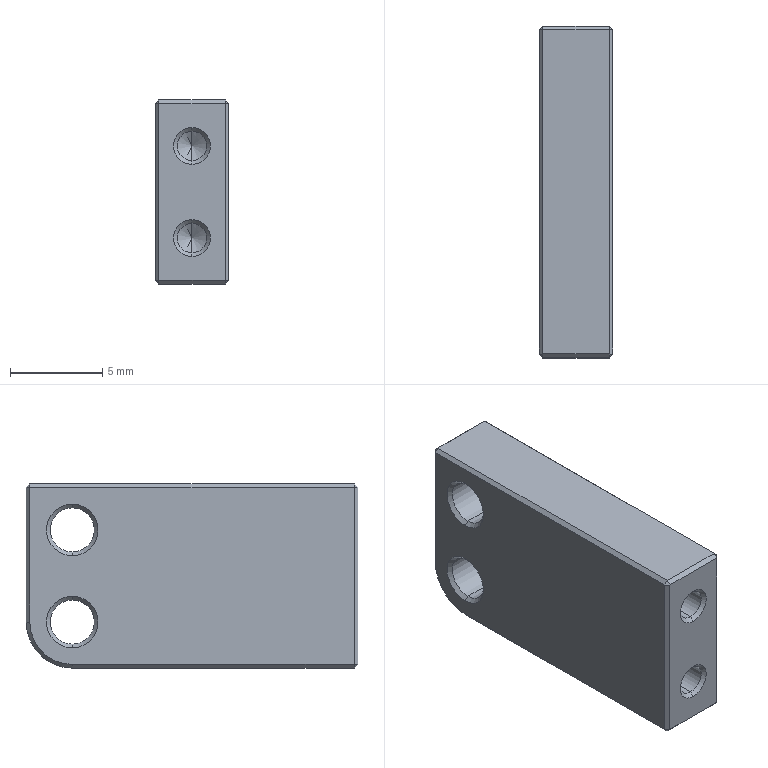Part | SolidWorks | features HoleWzd 2, Chamfer 1, Extrusion 1, Fillet 1 | 1 solid | 50 faces | box 4 x 18 x 10 mm | volume 638.389 mm3 | plane 23 | cone 18 | cylinder 9 | commonest cylinder face diameters 1.6 x4 2.4 x4 5 x1
STEP:
#1=CARTESIAN_POINT('',(0.2,15.5,-3.7));
#2=VERTEX_POINT('',#1);
#3=CARTESIAN_POINT('',(0.2,15.5,-1.3));
#4=VERTEX_POINT('',#3);
#5=CARTESIAN_POINT('',(0.2,15.5,-2.5));
#6=DIRECTION('',(-1.,0.,0.));
#7=DIRECTION('',(0.,0.,-1.));
#8=AXIS2_PLACEMENT_3D('',#5,#6,#7);
#9=CIRCLE('',#8,1.2);
#10=EDGE_CURVE('',#2,#4,#9,.T.);
#11=ORIENTED_EDGE('',*,*,#10,.F.);
#12=CARTESIAN_POINT('',(0.,15.5,-3.9));
#13=VERTEX_POINT('',#12);
#14=CARTESIAN_POINT('',(0.,15.5,-3.9));
#15=DIRECTION('',(-0.7071,0.,-0.7071));
#16=VECTOR('',#15,1000.);
#17=LINE('',#14,#16);
#18=EDGE_CURVE('',#2,#13,#17,.T.);
#19=ORIENTED_EDGE('',*,*,#18,.T.);
#20=CARTESIAN_POINT('',(0.,15.5,-1.1));
#21=VERTEX_POINT('',#20);
#22=CARTESIAN_POINT('',(0.,15.5,-2.5));
#23=DIRECTION('',(1.,0.,0.));
#24=DIRECTION('',(0.,0.,-1.));
#25=AXIS2_PLACEMENT_3D('',#22,#23,#24);
#26=CIRCLE('',#25,1.4);
#27=EDGE_CURVE('',#21,#13,#26,.T.);
#28=ORIENTED_EDGE('',*,*,#27,.F.);
#29=CARTESIAN_POINT('',(0.,15.5,-1.1));
#30=DIRECTION('',(-0.7071,0.,0.7071));
#31=VECTOR('',#30,1000.);
#32=LINE('',#29,#31);
#33=EDGE_CURVE('',#4,#21,#32,.T.);
#34=ORIENTED_EDGE('',*,*,#33,.F.);
#35=EDGE_LOOP('',(#11,#19,#28,#34));
#36=FACE_OUTER_BOUND('',#35,.T.);
#37=CARTESIAN_POINT('',(0.,15.5,-2.5));
#38=DIRECTION('',(-1.,0.,0.));
#39=DIRECTION('',(0.,0.,1.));
#40=AXIS2_PLACEMENT_3D('',#37,#38,#39);
#41=CONICAL_SURFACE('',#40,1.4,0.7854);
#42=ADVANCED_FACE('',(#36),#41,.F.);
#43=CARTESIAN_POINT('',(0.2,15.5,-8.7));
#44=VERTEX_POINT('',#43);
#45=CARTESIAN_POINT('',(0.2,15.5,-6.3));
#46=VERTEX_POINT('',#45);
#47=CARTESIAN_POINT('',(0.2,15.5,-7.5));
#48=DIRECTION('',(-1.,0.,0.));
#49=DIRECTION('',(0.,0.,-1.));
#50=AXIS2_PLACEMENT_3D('',#47,#48,#49);
#51=CIRCLE('',#50,1.2);
#52=EDGE_CURVE('',#44,#46,#51,.T.);
#53=ORIENTED_EDGE('',*,*,#52,.F.);
#54=CARTESIAN_POINT('',(0.,15.5,-8.9));
#55=VERTEX_POINT('',#54);
#56=CARTESIAN_POINT('',(0.,15.5,-8.9));
#57=DIRECTION('',(-0.7071,0.,-0.7071));
#58=VECTOR('',#57,1000.);
#59=LINE('',#56,#58);
#60=EDGE_CURVE('',#44,#55,#59,.T.);
#61=ORIENTED_EDGE('',*,*,#60,.T.);
#62=CARTESIAN_POINT('',(0.,15.5,-6.1));
#63=VERTEX_POINT('',#62);
#64=CARTESIAN_POINT('',(0.,15.5,-7.5));
#65=DIRECTION('',(1.,0.,0.));
#66=DIRECTION('',(0.,0.,-1.));
#67=AXIS2_PLACEMENT_3D('',#64,#65,#66);
#68=CIRCLE('',#67,1.4);
#69=EDGE_CURVE('',#63,#55,#68,.T.);
#70=ORIENTED_EDGE('',*,*,#69,.F.);
#71=CARTESIAN_POINT('',(0.,15.5,-6.1));
#72=DIRECTION('',(-0.7071,0.,0.7071));
#73=VECTOR('',#72,1000.);
#74=LINE('',#71,#73);
#75=EDGE_CURVE('',#46,#63,#74,.T.);
#76=ORIENTED_EDGE('',*,*,#75,.F.);
#77=EDGE_LOOP('',(#53,#61,#70,#76));
#78=FACE_OUTER_BOUND('',#77,.T.);
#79=CARTESIAN_POINT('',(0.,15.5,-7.5));
#80=DIRECTION('',(-1.,0.,0.));
#81=DIRECTION('',(0.,0.,1.));
#82=AXIS2_PLACEMENT_3D('',#79,#80,#81);
#83=CONICAL_SURFACE('',#82,1.4,0.7854);
#84=ADVANCED_FACE('',(#78),#83,.F.);
#85=CARTESIAN_POINT('',(2.,0.2,-1.7));
#86=VERTEX_POINT('',#85);
#87=CARTESIAN_POINT('',(2.,0.2,-3.3));
#88=VERTEX_POINT('',#87);
#89=CARTESIAN_POINT('',(2.,0.2,-2.5));
#90=DIRECTION('',(0.,-1.,0.));
#91=DIRECTION('',(0.,0.,-1.));
#92=AXIS2_PLACEMENT_3D('',#89,#90,#91);
#93=CIRCLE('',#92,0.8);
#94=EDGE_CURVE('',#86,#88,#93,.T.);
#95=ORIENTED_EDGE('',*,*,#94,.F.);
#96=CARTESIAN_POINT('',(2.,0.,-1.5));
#97=VERTEX_POINT('',#96);
#98=CARTESIAN_POINT('',(2.,0.2,-1.7));
#99=DIRECTION('',(0.,-0.7071,0.7071));
#100=VECTOR('',#99,1000.);
#101=LINE('',#98,#100);
#102=EDGE_CURVE('',#86,#97,#101,.T.);
#103=ORIENTED_EDGE('',*,*,#102,.T.);
#104=CARTESIAN_POINT('',(2.,0.,-3.5));
#105=VERTEX_POINT('',#104);
#106=CARTESIAN_POINT('',(2.,0.,-2.5));
#107=DIRECTION('',(0.,1.,0.));
#108=DIRECTION('',(0.,0.,-1.));
#109=AXIS2_PLACEMENT_3D('',#106,#107,#108);
#110=CIRCLE('',#109,1.);
#111=EDGE_CURVE('',#105,#97,#110,.T.);
#112=ORIENTED_EDGE('',*,*,#111,.F.);
#113=CARTESIAN_POINT('',(2.,0.2,-3.3));
#114=DIRECTION('',(0.,-0.7071,-0.7071));
#115=VECTOR('',#114,1000.);
#116=LINE('',#113,#115);
#117=EDGE_CURVE('',#88,#105,#116,.T.);
#118=ORIENTED_EDGE('',*,*,#117,.F.);
#119=EDGE_LOOP('',(#95,#103,#112,#118));
#120=FACE_OUTER_BOUND('',#119,.T.);
#121=CARTESIAN_POINT('',(2.,0.2,-2.5));
#122=DIRECTION('',(0.,-1.,0.));
#123=DIRECTION('',(0.,0.,-1.));
#124=AXIS2_PLACEMENT_3D('',#121,#122,#123);
#125=CONICAL_SURFACE('',#124,0.8,0.7854);
#126=ADVANCED_FACE('',(#120),#125,.F.);
#127=CARTESIAN_POINT('',(2.,0.2,-6.7));
#128=VERTEX_POINT('',#127);
#129=CARTESIAN_POINT('',(2.,0.2,-8.3));
#130=VERTEX_POINT('',#129);
#131=CARTESIAN_POINT('',(2.,0.2,-7.5));
#132=DIRECTION('',(0.,-1.,0.));
#133=DIRECTION('',(0.,0.,-1.));
#134=AXIS2_PLACEMENT_3D('',#131,#132,#133);
#135=CIRCLE('',#134,0.8);
#136=EDGE_CURVE('',#128,#130,#135,.T.);
#137=ORIENTED_EDGE('',*,*,#136,.F.);
#138=CARTESIAN_POINT('',(2.,0.,-6.5));
#139=VERTEX_POINT('',#138);
#140=CARTESIAN_POINT('',(2.,0.2,-6.7));
#141=DIRECTION('',(0.,-0.7071,0.7071));
#142=VECTOR('',#141,1000.);
#143=LINE('',#140,#142);
#144=EDGE_CURVE('',#128,#139,#143,.T.);
#145=ORIENTED_EDGE('',*,*,#144,.T.);
#146=CARTESIAN_POINT('',(2.,0.,-8.5));
#147=VERTEX_POINT('',#146);
#148=CARTESIAN_POINT('',(2.,0.,-7.5));
#149=DIRECTION('',(0.,1.,0.));
#150=DIRECTION('',(0.,0.,-1.));
#151=AXIS2_PLACEMENT_3D('',#148,#149,#150);
#152=CIRCLE('',#151,1.);
#153=EDGE_CURVE('',#147,#139,#152,.T.);
#154=ORIENTED_EDGE('',*,*,#153,.F.);
#155=CARTESIAN_POINT('',(2.,0.2,-8.3));
#156=DIRECTION('',(0.,-0.7071,-0.7071));
#157=VECTOR('',#156,1000.);
#158=LINE('',#155,#157);
#159=EDGE_CURVE('',#130,#147,#158,.T.);
#160=ORIENTED_EDGE('',*,*,#159,.F.);
#161=EDGE_LOOP('',(#137,#145,#154,#160));
#162=FACE_OUTER_BOUND('',#161,.T.);
#163=CARTESIAN_POINT('',(2.,0.2,-7.5));
#164=DIRECTION('',(0.,-1.,0.));
#165=DIRECTION('',(0.,0.,-1.));
#166=AXIS2_PLACEMENT_3D('',#163,#164,#165);
#167=CONICAL_SURFACE('',#166,0.8,0.7854);
#168=ADVANCED_FACE('',(#162),#167,.F.);
#169=CARTESIAN_POINT('',(2.,6.4,-1.7));
#170=VERTEX_POINT('',#169);
#171=CARTESIAN_POINT('',(2.,6.4,-3.3));
#172=VERTEX_POINT('',#171);
#173=CARTESIAN_POINT('',(2.,6.4,-2.5));
#174=DIRECTION('',(0.,-1.,0.));
#175=DIRECTION('',(0.,0.,-1.));
#176=AXIS2_PLACEMENT_3D('',#173,#174,#175);
#177=CIRCLE('',#176,0.8);
#178=EDGE_CURVE('',#170,#172,#177,.T.);
#179=ORIENTED_EDGE('',*,*,#178,.F.);
#180=CARTESIAN_POINT('',(2.,0.,-1.7));
#181=DIRECTION('',(0.,-1.,0.));
#182=VECTOR('',#181,1000.);
#183=LINE('',#180,#182);
#184=EDGE_CURVE('',#170,#86,#183,.T.);
#185=ORIENTED_EDGE('',*,*,#184,.T.);
#186=ORIENTED_EDGE('',*,*,#94,.T.);
#187=CARTESIAN_POINT('',(2.,0.,-3.3));
#188=DIRECTION('',(0.,-1.,0.));
#189=VECTOR('',#188,1000.);
#190=LINE('',#187,#189);
#191=EDGE_CURVE('',#172,#88,#190,.T.);
#192=ORIENTED_EDGE('',*,*,#191,.F.);
#193=EDGE_LOOP('',(#179,#185,#186,#192));
#194=FACE_OUTER_BOUND('',#193,.T.);
#195=CARTESIAN_POINT('',(2.,0.,-2.5));
#196=DIRECTION('',(0.,-1.,0.));
#197=DIRECTION('',(0.,0.,-1.));
#198=AXIS2_PLACEMENT_3D('',#195,#196,#197);
#199=CYLINDRICAL_SURFACE('',#198,0.8);
#200=ADVANCED_FACE('',(#194),#199,.F.);
#201=CARTESIAN_POINT('',(2.,6.881,-2.5));
#202=VERTEX_POINT('',#201);
#203=CARTESIAN_POINT('',(2.,6.4,-3.3));
#204=DIRECTION('',(0.,-0.515,-0.8572));
#205=VECTOR('',#204,1000.);
#206=LINE('',#203,#205);
#207=EDGE_CURVE('',#202,#172,#206,.T.);
#208=ORIENTED_EDGE('',*,*,#207,.F.);
#209=CARTESIAN_POINT('',(2.,6.4,-1.7));
#210=DIRECTION('',(0.,-0.515,0.8572));
#211=VECTOR('',#210,1000.);
#212=LINE('',#209,#211);
#213=EDGE_CURVE('',#202,#170,#212,.T.);
#214=ORIENTED_EDGE('',*,*,#213,.T.);
#215=ORIENTED_EDGE('',*,*,#178,.T.);
#216=EDGE_LOOP('',(#208,#214,#215));
#217=FACE_OUTER_BOUND('',#216,.T.);
#218=CARTESIAN_POINT('',(2.,6.4,-2.5));
#219=DIRECTION('',(0.,-1.,0.));
#220=DIRECTION('',(0.,0.,-1.));
#221=AXIS2_PLACEMENT_3D('',#218,#219,#220);
#222=CONICAL_SURFACE('',#221,0.8,1.03);
#223=ADVANCED_FACE('',(#217),#222,.F.);
#224=CARTESIAN_POINT('',(2.,6.4,-6.7));
#225=VERTEX_POINT('',#224);
#226=CARTESIAN_POINT('',(2.,6.4,-8.3));
#227=VERTEX_POINT('',#226);
#228=CARTESIAN_POINT('',(2.,6.4,-7.5));
#229=DIRECTION('',(0.,-1.,0.));
#230=DIRECTION('',(0.,0.,-1.));
#231=AXIS2_PLACEMENT_3D('',#228,#229,#230);
#232=CIRCLE('',#231,0.8);
#233=EDGE_CURVE('',#225,#227,#232,.T.);
#234=ORIENTED_EDGE('',*,*,#233,.F.);
#235=CARTESIAN_POINT('',(2.,0.,-6.7));
#236=DIRECTION('',(0.,-1.,0.));
#237=VECTOR('',#236,1000.);
#238=LINE('',#235,#237);
#239=EDGE_CURVE('',#225,#128,#238,.T.);
#240=ORIENTED_EDGE('',*,*,#239,.T.);
#241=ORIENTED_EDGE('',*,*,#136,.T.);
#242=CARTESIAN_POINT('',(2.,0.,-8.3));
#243=DIRECTION('',(0.,-1.,0.));
#244=VECTOR('',#243,1000.);
#245=LINE('',#242,#244);
#246=EDGE_CURVE('',#227,#130,#245,.T.);
#247=ORIENTED_EDGE('',*,*,#246,.F.);
#248=EDGE_LOOP('',(#234,#240,#241,#247));
#249=FACE_OUTER_BOUND('',#248,.T.);
#250=CARTESIAN_POINT('',(2.,0.,-7.5));
#251=DIRECTION('',(0.,-1.,0.));
#252=DIRECTION('',(0.,0.,-1.));
#253=AXIS2_PLACEMENT_3D('',#250,#251,#252);
#254=CYLINDRICAL_SURFACE('',#253,0.8);
#255=ADVANCED_FACE('',(#249),#254,.F.);
#256=CARTESIAN_POINT('',(2.,6.881,-7.5));
#257=VERTEX_POINT('',#256);
#258=CARTESIAN_POINT('',(2.,6.4,-8.3));
#259=DIRECTION('',(0.,-0.515,-0.8572));
#260=VECTOR('',#259,1000.);
#261=LINE('',#258,#260);
#262=EDGE_CURVE('',#257,#227,#261,.T.);
#263=ORIENTED_EDGE('',*,*,#262,.F.);
#264=CARTESIAN_POINT('',(2.,6.4,-6.7));
#265=DIRECTION('',(0.,-0.515,0.8572));
#266=VECTOR('',#265,1000.);
#267=LINE('',#264,#266);
#268=EDGE_CURVE('',#257,#225,#267,.T.);
#269=ORIENTED_EDGE('',*,*,#268,.T.);
#270=ORIENTED_EDGE('',*,*,#233,.T.);
#271=EDGE_LOOP('',(#263,#269,#270));
#272=FACE_OUTER_BOUND('',#271,.T.);
#273=CARTESIAN_POINT('',(2.,6.4,-7.5));
#274=DIRECTION('',(0.,-1.,0.));
#275=DIRECTION('',(0.,0.,-1.));
#276=AXIS2_PLACEMENT_3D('',#273,#274,#275);
#277=CONICAL_SURFACE('',#276,0.8,1.03);
#278=ADVANCED_FACE('',(#272),#277,.F.);
#279=CARTESIAN_POINT('',(2.95,15.5,-1.3));
#280=VERTEX_POINT('',#279);
#281=CARTESIAN_POINT('',(2.95,15.5,-3.7));
#282=VERTEX_POINT('',#281);
#283=CARTESIAN_POINT('',(2.95,15.5,-2.5));
#284=DIRECTION('',(1.,0.,0.));
#285=DIRECTION('',(0.,0.,-1.));
#286=AXIS2_PLACEMENT_3D('',#283,#284,#285);
#287=CIRCLE('',#286,1.2);
#288=EDGE_CURVE('',#280,#282,#287,.T.);
#289=ORIENTED_EDGE('',*,*,#288,.F.);
#290=CARTESIAN_POINT('',(4.,15.5,-0.25));
#291=VERTEX_POINT('',#290);
#292=CARTESIAN_POINT('',(4.,15.5,-0.25));
#293=DIRECTION('',(0.7071,0.,0.7071));
#294=VECTOR('',#293,1000.);
#295=LINE('',#292,#294);
#296=EDGE_CURVE('',#280,#291,#295,.T.);
#297=ORIENTED_EDGE('',*,*,#296,.T.);
#298=CARTESIAN_POINT('',(4.,15.5,-4.75));
#299=VERTEX_POINT('',#298);
#300=CARTESIAN_POINT('',(4.,15.5,-2.5));
#301=DIRECTION('',(1.,0.,0.));
#302=DIRECTION('',(0.,0.,-1.));
#303=AXIS2_PLACEMENT_3D('',#300,#301,#302);
#304=CIRCLE('',#303,2.25);
#305=EDGE_CURVE('',#291,#299,#304,.T.);
#306=ORIENTED_EDGE('',*,*,#305,.T.);
#307=CARTESIAN_POINT('',(4.,15.5,-4.75));
#308=DIRECTION('',(0.7071,0.,-0.7071));
#309=VECTOR('',#308,1000.);
#310=LINE('',#307,#309);
#311=EDGE_CURVE('',#282,#299,#310,.T.);
#312=ORIENTED_EDGE('',*,*,#311,.F.);
#313=EDGE_LOOP('',(#289,#297,#306,#312));
#314=FACE_OUTER_BOUND('',#313,.T.);
#315=CARTESIAN_POINT('',(4.,15.5,-2.5));
#316=DIRECTION('',(1.,0.,0.));
#317=DIRECTION('',(0.,0.,-1.));
#318=AXIS2_PLACEMENT_3D('',#315,#316,#317);
#319=CONICAL_SURFACE('',#318,2.25,0.7854);
#320=ADVANCED_FACE('',(#314),#319,.F.);
#321=ORIENTED_EDGE('',*,*,#10,.T.);
#322=CARTESIAN_POINT('',(4.,15.5,-1.3));
#323=DIRECTION('',(1.,0.,0.));
#324=VECTOR('',#323,1000.);
#325=LINE('',#322,#324);
#326=EDGE_CURVE('',#4,#280,#325,.T.);
#327=ORIENTED_EDGE('',*,*,#326,.T.);
#328=ORIENTED_EDGE('',*,*,#288,.T.);
#329=CARTESIAN_POINT('',(4.,15.5,-3.7));
#330=DIRECTION('',(1.,0.,0.));
#331=VECTOR('',#330,1000.);
#332=LINE('',#329,#331);
#333=EDGE_CURVE('',#2,#282,#332,.T.);
#334=ORIENTED_EDGE('',*,*,#333,.F.);
#335=EDGE_LOOP('',(#321,#327,#328,#334));
#336=FACE_OUTER_BOUND('',#335,.T.);
#337=CARTESIAN_POINT('',(4.,15.5,-2.5));
#338=DIRECTION('',(1.,0.,0.));
#339=DIRECTION('',(0.,0.,-1.));
#340=AXIS2_PLACEMENT_3D('',#337,#338,#339);
#341=CYLINDRICAL_SURFACE('',#340,1.2);
#342=ADVANCED_FACE('',(#336),#341,.F.);
#343=CARTESIAN_POINT('',(2.95,15.5,-6.3));
#344=VERTEX_POINT('',#343);
#345=CARTESIAN_POINT('',(2.95,15.5,-8.7));
#346=VERTEX_POINT('',#345);
#347=CARTESIAN_POINT('',(2.95,15.5,-7.5));
#348=DIRECTION('',(1.,0.,0.));
#349=DIRECTION('',(0.,0.,-1.));
#350=AXIS2_PLACEMENT_3D('',#347,#348,#349);
#351=CIRCLE('',#350,1.2);
#352=EDGE_CURVE('',#344,#346,#351,.T.);
#353=ORIENTED_EDGE('',*,*,#352,.F.);
#354=CARTESIAN_POINT('',(4.,15.5,-5.25));
#355=VERTEX_POINT('',#354);
#356=CARTESIAN_POINT('',(4.,15.5,-5.25));
#357=DIRECTION('',(0.7071,0.,0.7071));
#358=VECTOR('',#357,1000.);
#359=LINE('',#356,#358);
#360=EDGE_CURVE('',#344,#355,#359,.T.);
#361=ORIENTED_EDGE('',*,*,#360,.T.);
#362=CARTESIAN_POINT('',(4.,15.5,-9.75));
#363=VERTEX_POINT('',#362);
#364=CARTESIAN_POINT('',(4.,15.5,-7.5));
#365=DIRECTION('',(1.,0.,0.));
#366=DIRECTION('',(0.,0.,-1.));
#367=AXIS2_PLACEMENT_3D('',#364,#365,#366);
#368=CIRCLE('',#367,2.25);
#369=EDGE_CURVE('',#355,#363,#368,.T.);
#370=ORIENTED_EDGE('',*,*,#369,.T.);
#371=CARTESIAN_POINT('',(4.,15.5,-9.75));
#372=DIRECTION('',(0.7071,0.,-0.7071));
#373=VECTOR('',#372,1000.);
#374=LINE('',#371,#373);
#375=EDGE_CURVE('',#346,#363,#374,.T.);
#376=ORIENTED_EDGE('',*,*,#375,.F.);
#377=EDGE_LOOP('',(#353,#361,#370,#376));
#378=FACE_OUTER_BOUND('',#377,.T.);
#379=CARTESIAN_POINT('',(4.,15.5,-7.5));
#380=DIRECTION('',(1.,0.,0.));
#381=DIRECTION('',(0.,0.,-1.));
#382=AXIS2_PLACEMENT_3D('',#379,#380,#381);
#383=CONICAL_SURFACE('',#382,2.25,0.7854);
#384=ADVANCED_FACE('',(#378),#383,.F.);
#385=ORIENTED_EDGE('',*,*,#52,.T.);
#386=CARTESIAN_POINT('',(4.,15.5,-6.3));
#387=DIRECTION('',(1.,0.,0.));
#388=VECTOR('',#387,1000.);
#389=LINE('',#386,#388);
#390=EDGE_CURVE('',#46,#344,#389,.T.);
#391=ORIENTED_EDGE('',*,*,#390,.T.);
#392=ORIENTED_EDGE('',*,*,#352,.T.);
#393=CARTESIAN_POINT('',(4.,15.5,-8.7));
#394=DIRECTION('',(1.,0.,0.));
#395=VECTOR('',#394,1000.);
#396=LINE('',#393,#395);
#397=EDGE_CURVE('',#44,#346,#396,.T.);
#398=ORIENTED_EDGE('',*,*,#397,.F.);
#399=EDGE_LOOP('',(#385,#391,#392,#398));
#400=FACE_OUTER_BOUND('',#399,.T.);
#401=CARTESIAN_POINT('',(4.,15.5,-7.5));
#402=DIRECTION('',(1.,0.,0.));
#403=DIRECTION('',(0.,0.,-1.));
#404=AXIS2_PLACEMENT_3D('',#401,#402,#403);
#405=CYLINDRICAL_SURFACE('',#404,1.2);
#406=ADVANCED_FACE('',(#400),#405,.F.);
#407=CARTESIAN_POINT('',(4.,0.2,-0.2));
#408=VERTEX_POINT('',#407);
#409=CARTESIAN_POINT('',(4.,0.2,-9.8));
#410=VERTEX_POINT('',#409);
#411=CARTESIAN_POINT('',(4.,0.2,-10.));
#412=DIRECTION('',(0.,0.,-1.));
#413=VECTOR('',#412,1000.);
#414=LINE('',#411,#413);
#415=EDGE_CURVE('',#408,#410,#414,.T.);
#416=ORIENTED_EDGE('',*,*,#415,.T.);
#417=CARTESIAN_POINT('',(4.,15.5,-9.8));
#418=VERTEX_POINT('',#417);
#419=CARTESIAN_POINT('',(4.,18.,-9.8));
#420=DIRECTION('',(0.,1.,0.));
#421=VECTOR('',#420,1000.);
#422=LINE('',#419,#421);
#423=EDGE_CURVE('',#410,#418,#422,.T.);
#424=ORIENTED_EDGE('',*,*,#423,.T.);
#425=CARTESIAN_POINT('',(4.,17.8,-7.5));
#426=VERTEX_POINT('',#425);
#427=CARTESIAN_POINT('',(4.,15.5,-7.5));
#428=DIRECTION('',(1.,0.,0.));
#429=DIRECTION('',(0.,0.,1.));
#430=AXIS2_PLACEMENT_3D('',#427,#428,#429);
#431=CIRCLE('',#430,2.3);
#432=EDGE_CURVE('',#418,#426,#431,.T.);
#433=ORIENTED_EDGE('',*,*,#432,.T.);
#434=CARTESIAN_POINT('',(4.,17.8,-0.2));
#435=VERTEX_POINT('',#434);
#436=CARTESIAN_POINT('',(4.,17.8,0.));
#437=DIRECTION('',(0.,0.,1.));
#438=VECTOR('',#437,1000.);
#439=LINE('',#436,#438);
#440=EDGE_CURVE('',#426,#435,#439,.T.);
#441=ORIENTED_EDGE('',*,*,#440,.T.);
#442=CARTESIAN_POINT('',(4.,18.,-0.2));
#443=DIRECTION('',(0.,-1.,0.));
#444=VECTOR('',#443,1000.);
#445=LINE('',#442,#444);
#446=EDGE_CURVE('',#435,#408,#445,.T.);
#447=ORIENTED_EDGE('',*,*,#446,.T.);
#448=EDGE_LOOP('',(#416,#424,#433,#441,#447));
#449=FACE_OUTER_BOUND('',#448,.T.);
#450=CARTESIAN_POINT('',(4.,15.5,-2.5));
#451=DIRECTION('',(1.,0.,0.));
#452=DIRECTION('',(0.,0.,-1.));
#453=AXIS2_PLACEMENT_3D('',#450,#451,#452);
#454=CIRCLE('',#453,2.25);
#455=EDGE_CURVE('',#299,#291,#454,.T.);
#456=ORIENTED_EDGE('',*,*,#455,.F.);
#457=ORIENTED_EDGE('',*,*,#305,.F.);
#458=EDGE_LOOP('',(#456,#457));
#459=FACE_BOUND('',#458,.T.);
#460=CARTESIAN_POINT('',(4.,15.5,-7.5));
#461=DIRECTION('',(1.,0.,0.));
#462=DIRECTION('',(0.,0.,-1.));
#463=AXIS2_PLACEMENT_3D('',#460,#461,#462);
#464=CIRCLE('',#463,2.25);
#465=EDGE_CURVE('',#363,#355,#464,.T.);
#466=ORIENTED_EDGE('',*,*,#465,.F.);
#467=ORIENTED_EDGE('',*,*,#369,.F.);
#468=EDGE_LOOP('',(#466,#467));
#469=FACE_BOUND('',#468,.T.);
#470=CARTESIAN_POINT('',(4.,18.,0.));
#471=DIRECTION('',(-1.,0.,0.));
#472=DIRECTION('',(0.,0.,1.));
#473=AXIS2_PLACEMENT_3D('',#470,#471,#472);
#474=PLANE('',#473);
#475=ADVANCED_FACE('',(#449,#459,#469),#474,.F.);
#476=CARTESIAN_POINT('',(0.,0.2,-9.8));
#477=VERTEX_POINT('',#476);
#478=CARTESIAN_POINT('',(0.,0.2,-0.2));
#479=VERTEX_POINT('',#478);
#480=CARTESIAN_POINT('',(0.,0.2,0.));
#481=DIRECTION('',(0.,0.,1.));
#482=VECTOR('',#481,1000.);
#483=LINE('',#480,#482);
#484=EDGE_CURVE('',#477,#479,#483,.T.);
#485=ORIENTED_EDGE('',*,*,#484,.T.);
#486=CARTESIAN_POINT('',(0.,17.8,-0.2));
#487=VERTEX_POINT('',#486);
#488=CARTESIAN_POINT('',(0.,18.,-0.2));
#489=DIRECTION('',(0.,1.,0.));
#490=VECTOR('',#489,1000.);
#491=LINE('',#488,#490);
#492=EDGE_CURVE('',#479,#487,#491,.T.);
#493=ORIENTED_EDGE('',*,*,#492,.T.);
#494=CARTESIAN_POINT('',(0.,17.8,-7.5));
#495=VERTEX_POINT('',#494);
#496=CARTESIAN_POINT('',(0.,17.8,0.));
#497=DIRECTION('',(0.,0.,-1.));
#498=VECTOR('',#497,1000.);
#499=LINE('',#496,#498);
#500=EDGE_CURVE('',#487,#495,#499,.T.);
#501=ORIENTED_EDGE('',*,*,#500,.T.);
#502=CARTESIAN_POINT('',(0.,15.5,-9.8));
#503=VERTEX_POINT('',#502);
#504=CARTESIAN_POINT('',(0.,15.5,-7.5));
#505=DIRECTION('',(-1.,0.,0.));
#506=DIRECTION('',(0.,0.,-1.));
#507=AXIS2_PLACEMENT_3D('',#504,#505,#506);
#508=CIRCLE('',#507,2.3);
#509=EDGE_CURVE('',#495,#503,#508,.T.);
#510=ORIENTED_EDGE('',*,*,#509,.T.);
#511=CARTESIAN_POINT('',(0.,18.,-9.8));
#512=DIRECTION('',(0.,-1.,0.));
#513=VECTOR('',#512,1000.);
#514=LINE('',#511,#513);
#515=EDGE_CURVE('',#503,#477,#514,.T.);
#516=ORIENTED_EDGE('',*,*,#515,.T.);
#517=EDGE_LOOP('',(#485,#493,#501,#510,#516));
#518=FACE_OUTER_BOUND('',#517,.T.);
#519=ORIENTED_EDGE('',*,*,#69,.T.);
#520=CARTESIAN_POINT('',(0.,15.5,-7.5));
#521=DIRECTION('',(1.,0.,0.));
#522=DIRECTION('',(0.,0.,-1.));
#523=AXIS2_PLACEMENT_3D('',#520,#521,#522);
#524=CIRCLE('',#523,1.4);
#525=EDGE_CURVE('',#55,#63,#524,.T.);
#526=ORIENTED_EDGE('',*,*,#525,.T.);
#527=EDGE_LOOP('',(#519,#526));
#528=FACE_BOUND('',#527,.T.);
#529=ORIENTED_EDGE('',*,*,#27,.T.);
#530=CARTESIAN_POINT('',(0.,15.5,-2.5));
#531=DIRECTION('',(1.,0.,0.));
#532=DIRECTION('',(0.,0.,-1.));
#533=AXIS2_PLACEMENT_3D('',#530,#531,#532);
#534=CIRCLE('',#533,1.4);
#535=EDGE_CURVE('',#13,#21,#534,.T.);
#536=ORIENTED_EDGE('',*,*,#535,.T.);
#537=EDGE_LOOP('',(#529,#536));
#538=FACE_BOUND('',#537,.T.);
#539=CARTESIAN_POINT('',(0.,18.,0.));
#540=DIRECTION('',(1.,0.,0.));
#541=DIRECTION('',(0.,0.,-1.));
#542=AXIS2_PLACEMENT_3D('',#539,#540,#541);
#543=PLANE('',#542);
#544=ADVANCED_FACE('',(#518,#528,#538),#543,.F.);
#545=CARTESIAN_POINT('',(3.8,0.2,0.));
#546=VERTEX_POINT('',#545);
#547=CARTESIAN_POINT('',(3.8,17.8,0.));
#548=VERTEX_POINT('',#547);
#549=CARTESIAN_POINT('',(3.8,18.,0.));
#550=DIRECTION('',(0.,1.,0.));
#551=VECTOR('',#550,1000.);
#552=LINE('',#549,#551);
#553=EDGE_CURVE('',#546,#548,#552,.T.);
#554=ORIENTED_EDGE('',*,*,#553,.T.);
#555=CARTESIAN_POINT('',(0.2,17.8,0.));
#556=VERTEX_POINT('',#555);
#557=CARTESIAN_POINT('',(0.,17.8,0.));
#558=DIRECTION('',(-1.,0.,0.));
#559=VECTOR('',#558,1000.);
#560=LINE('',#557,#559);
#561=EDGE_CURVE('',#548,#556,#560,.T.);
#562=ORIENTED_EDGE('',*,*,#561,.T.);
#563=CARTESIAN_POINT('',(0.2,0.2,0.));
#564=VERTEX_POINT('',#563);
#565=CARTESIAN_POINT('',(0.2,18.,0.));
#566=DIRECTION('',(0.,-1.,0.));
#567=VECTOR('',#566,1000.);
#568=LINE('',#565,#567);
#569=EDGE_CURVE('',#556,#564,#568,.T.);
#570=ORIENTED_EDGE('',*,*,#569,.T.);
#571=CARTESIAN_POINT('',(4.,0.2,0.));
#572=DIRECTION('',(1.,0.,0.));
#573=VECTOR('',#572,1000.);
#574=LINE('',#571,#573);
#575=EDGE_CURVE('',#564,#546,#574,.T.);
#576=ORIENTED_EDGE('',*,*,#575,.T.);
#577=EDGE_LOOP('',(#554,#562,#570,#576));
#578=FACE_OUTER_BOUND('',#577,.T.);
#579=CARTESIAN_POINT('',(0.,18.,0.));
#580=DIRECTION('',(0.,0.,-1.));
#581=DIRECTION('',(-1.,0.,0.));
#582=AXIS2_PLACEMENT_3D('',#579,#580,#581);
#583=PLANE('',#582);
#584=ADVANCED_FACE('',(#578),#583,.F.);
#585=CARTESIAN_POINT('',(0.2,15.5,-10.));
#586=VERTEX_POINT('',#585);
#587=CARTESIAN_POINT('',(3.8,15.5,-10.));
#588=VERTEX_POINT('',#587);
#589=CARTESIAN_POINT('',(0.,15.5,-10.));
#590=DIRECTION('',(1.,0.,0.));
#591=VECTOR('',#590,1000.);
#592=LINE('',#589,#591);
#593=EDGE_CURVE('',#586,#588,#592,.T.);
#594=ORIENTED_EDGE('',*,*,#593,.T.);
#595=CARTESIAN_POINT('',(3.8,0.2,-10.));
#596=VERTEX_POINT('',#595);
#597=CARTESIAN_POINT('',(3.8,18.,-10.));
#598=DIRECTION('',(0.,-1.,0.));
#599=VECTOR('',#598,1000.);
#600=LINE('',#597,#599);
#601=EDGE_CURVE('',#588,#596,#600,.T.);
#602=ORIENTED_EDGE('',*,*,#601,.T.);
#603=CARTESIAN_POINT('',(0.2,0.2,-10.));
#604=VERTEX_POINT('',#603);
#605=CARTESIAN_POINT('',(0.,0.2,-10.));
#606=DIRECTION('',(-1.,0.,0.));
#607=VECTOR('',#606,1000.);
#608=LINE('',#605,#607);
#609=EDGE_CURVE('',#596,#604,#608,.T.);
#610=ORIENTED_EDGE('',*,*,#609,.T.);
#611=CARTESIAN_POINT('',(0.2,18.,-10.));
#612=DIRECTION('',(0.,1.,0.));
#613=VECTOR('',#612,1000.);
#614=LINE('',#611,#613);
#615=EDGE_CURVE('',#604,#586,#614,.T.);
#616=ORIENTED_EDGE('',*,*,#615,.T.);
#617=EDGE_LOOP('',(#594,#602,#610,#616));
#618=FACE_OUTER_BOUND('',#617,.T.);
#619=CARTESIAN_POINT('',(0.,18.,-10.));
#620=DIRECTION('',(0.,0.,1.));
#621=DIRECTION('',(1.,0.,0.));
#622=AXIS2_PLACEMENT_3D('',#619,#620,#621);
#623=PLANE('',#622);
#624=ADVANCED_FACE('',(#618),#623,.F.);
#625=CARTESIAN_POINT('',(0.2,18.,-0.2));
#626=VERTEX_POINT('',#625);
#627=CARTESIAN_POINT('',(3.8,18.,-0.2));
#628=VERTEX_POINT('',#627);
#629=CARTESIAN_POINT('',(0.,18.,-0.2));
#630=DIRECTION('',(1.,0.,0.));
#631=VECTOR('',#630,1000.);
#632=LINE('',#629,#631);
#633=EDGE_CURVE('',#626,#628,#632,.T.);
#634=ORIENTED_EDGE('',*,*,#633,.T.);
#635=CARTESIAN_POINT('',(3.8,18.,-7.5));
#636=VERTEX_POINT('',#635);
#637=CARTESIAN_POINT('',(3.8,18.,0.));
#638=DIRECTION('',(0.,0.,-1.));
#639=VECTOR('',#638,1000.);
#640=LINE('',#637,#639);
#641=EDGE_CURVE('',#628,#636,#640,.T.);
#642=ORIENTED_EDGE('',*,*,#641,.T.);
#643=CARTESIAN_POINT('',(0.2,18.,-7.5));
#644=VERTEX_POINT('',#643);
#645=CARTESIAN_POINT('',(0.,18.,-7.5));
#646=DIRECTION('',(-1.,0.,0.));
#647=VECTOR('',#646,1000.);
#648=LINE('',#645,#647);
#649=EDGE_CURVE('',#636,#644,#648,.T.);
#650=ORIENTED_EDGE('',*,*,#649,.T.);
#651=CARTESIAN_POINT('',(0.2,18.,0.));
#652=DIRECTION('',(0.,0.,1.));
#653=VECTOR('',#652,1000.);
#654=LINE('',#651,#653);
#655=EDGE_CURVE('',#644,#626,#654,.T.);
#656=ORIENTED_EDGE('',*,*,#655,.T.);
#657=EDGE_LOOP('',(#634,#642,#650,#656));
#658=FACE_OUTER_BOUND('',#657,.T.);
#659=CARTESIAN_POINT('',(0.,18.,0.));
#660=DIRECTION('',(0.,-1.,0.));
#661=DIRECTION('',(0.,0.,-1.));
#662=AXIS2_PLACEMENT_3D('',#659,#660,#661);
#663=PLANE('',#662);
#664=ADVANCED_FACE('',(#658),#663,.F.);
#665=ORIENTED_EDGE('',*,*,#153,.T.);
#666=CARTESIAN_POINT('',(2.,0.,-7.5));
#667=DIRECTION('',(0.,1.,0.));
#668=DIRECTION('',(0.,0.,-1.));
#669=AXIS2_PLACEMENT_3D('',#666,#667,#668);
#670=CIRCLE('',#669,1.);
#671=EDGE_CURVE('',#139,#147,#670,.T.);
#672=ORIENTED_EDGE('',*,*,#671,.T.);
#673=EDGE_LOOP('',(#665,#672));
#674=FACE_BOUND('',#673,.T.);
#675=ORIENTED_EDGE('',*,*,#111,.T.);
#676=CARTESIAN_POINT('',(2.,0.,-2.5));
#677=DIRECTION('',(0.,1.,0.));
#678=DIRECTION('',(0.,0.,-1.));
#679=AXIS2_PLACEMENT_3D('',#676,#677,#678);
#680=CIRCLE('',#679,1.);
#681=EDGE_CURVE('',#97,#105,#680,.T.);
#682=ORIENTED_EDGE('',*,*,#681,.T.);
#683=EDGE_LOOP('',(#675,#682));
#684=FACE_BOUND('',#683,.T.);
#685=CARTESIAN_POINT('',(0.2,0.,-9.8));
#686=VERTEX_POINT('',#685);
#687=CARTESIAN_POINT('',(3.8,0.,-9.8));
#688=VERTEX_POINT('',#687);
#689=CARTESIAN_POINT('',(4.,0.,-9.8));
#690=DIRECTION('',(1.,0.,0.));
#691=VECTOR('',#690,1000.);
#692=LINE('',#689,#691);
#693=EDGE_CURVE('',#686,#688,#692,.T.);
#694=ORIENTED_EDGE('',*,*,#693,.T.);
#695=CARTESIAN_POINT('',(3.8,0.,-0.2));
#696=VERTEX_POINT('',#695);
#697=CARTESIAN_POINT('',(3.8,0.,0.));
#698=DIRECTION('',(0.,0.,1.));
#699=VECTOR('',#698,1000.);
#700=LINE('',#697,#699);
#701=EDGE_CURVE('',#688,#696,#700,.T.);
#702=ORIENTED_EDGE('',*,*,#701,.T.);
#703=CARTESIAN_POINT('',(0.2,0.,-0.2));
#704=VERTEX_POINT('',#703);
#705=CARTESIAN_POINT('',(0.,0.,-0.2));
#706=DIRECTION('',(-1.,0.,0.));
#707=VECTOR('',#706,1000.);
#708=LINE('',#705,#707);
#709=EDGE_CURVE('',#696,#704,#708,.T.);
#710=ORIENTED_EDGE('',*,*,#709,.T.);
#711=CARTESIAN_POINT('',(0.2,0.,-10.));
#712=DIRECTION('',(0.,0.,-1.));
#713=VECTOR('',#712,1000.);
#714=LINE('',#711,#713);
#715=EDGE_CURVE('',#704,#686,#714,.T.);
#716=ORIENTED_EDGE('',*,*,#715,.T.);
#717=EDGE_LOOP('',(#694,#702,#710,#716));
#718=FACE_OUTER_BOUND('',#717,.T.);
#719=CARTESIAN_POINT('',(0.,0.,0.));
#720=DIRECTION('',(0.,-1.,0.));
#721=DIRECTION('',(0.,0.,-1.));
#722=AXIS2_PLACEMENT_3D('',#719,#720,#721);
#723=PLANE('',#722);
#724=ADVANCED_FACE('',(#674,#684,#718),#723,.T.);
#725=ORIENTED_EDGE('',*,*,#390,.F.);
#726=CARTESIAN_POINT('',(0.2,15.5,-7.5));
#727=DIRECTION('',(-1.,0.,0.));
#728=DIRECTION('',(0.,0.,-1.));
#729=AXIS2_PLACEMENT_3D('',#726,#727,#728);
#730=CIRCLE('',#729,1.2);
#731=EDGE_CURVE('',#46,#44,#730,.T.);
#732=ORIENTED_EDGE('',*,*,#731,.T.);
#733=ORIENTED_EDGE('',*,*,#397,.T.);
#734=CARTESIAN_POINT('',(2.95,15.5,-7.5));
#735=DIRECTION('',(1.,0.,0.));
#736=DIRECTION('',(0.,0.,-1.));
#737=AXIS2_PLACEMENT_3D('',#734,#735,#736);
#738=CIRCLE('',#737,1.2);
#739=EDGE_CURVE('',#346,#344,#738,.T.);
#740=ORIENTED_EDGE('',*,*,#739,.T.);
#741=EDGE_LOOP('',(#725,#732,#733,#740));
#742=FACE_OUTER_BOUND('',#741,.T.);
#743=CARTESIAN_POINT('',(4.,15.5,-7.5));
#744=DIRECTION('',(1.,0.,0.));
#745=DIRECTION('',(0.,0.,-1.));
#746=AXIS2_PLACEMENT_3D('',#743,#744,#745);
#747=CYLINDRICAL_SURFACE('',#746,1.2);
#748=ADVANCED_FACE('',(#742),#747,.F.);
#749=ORIENTED_EDGE('',*,*,#360,.F.);
#750=ORIENTED_EDGE('',*,*,#739,.F.);
#751=ORIENTED_EDGE('',*,*,#375,.T.);
#752=ORIENTED_EDGE('',*,*,#465,.T.);
#753=EDGE_LOOP('',(#749,#750,#751,#752));
#754=FACE_OUTER_BOUND('',#753,.T.);
#755=CARTESIAN_POINT('',(4.,15.5,-7.5));
#756=DIRECTION('',(1.,0.,0.));
#757=DIRECTION('',(0.,0.,-1.));
#758=AXIS2_PLACEMENT_3D('',#755,#756,#757);
#759=CONICAL_SURFACE('',#758,2.25,0.7854);
#760=ADVANCED_FACE('',(#754),#759,.F.);
#761=ORIENTED_EDGE('',*,*,#326,.F.);
#762=CARTESIAN_POINT('',(0.2,15.5,-2.5));
#763=DIRECTION('',(-1.,0.,0.));
#764=DIRECTION('',(0.,0.,-1.));
#765=AXIS2_PLACEMENT_3D('',#762,#763,#764);
#766=CIRCLE('',#765,1.2);
#767=EDGE_CURVE('',#4,#2,#766,.T.);
#768=ORIENTED_EDGE('',*,*,#767,.T.);
#769=ORIENTED_EDGE('',*,*,#333,.T.);
#770=CARTESIAN_POINT('',(2.95,15.5,-2.5));
#771=DIRECTION('',(1.,0.,0.));
#772=DIRECTION('',(0.,0.,-1.));
#773=AXIS2_PLACEMENT_3D('',#770,#771,#772);
#774=CIRCLE('',#773,1.2);
#775=EDGE_CURVE('',#282,#280,#774,.T.);
#776=ORIENTED_EDGE('',*,*,#775,.T.);
#777=EDGE_LOOP('',(#761,#768,#769,#776));
#778=FACE_OUTER_BOUND('',#777,.T.);
#779=CARTESIAN_POINT('',(4.,15.5,-2.5));
#780=DIRECTION('',(1.,0.,0.));
#781=DIRECTION('',(0.,0.,-1.));
#782=AXIS2_PLACEMENT_3D('',#779,#780,#781);
#783=CYLINDRICAL_SURFACE('',#782,1.2);
#784=ADVANCED_FACE('',(#778),#783,.F.);
#785=ORIENTED_EDGE('',*,*,#296,.F.);
#786=ORIENTED_EDGE('',*,*,#775,.F.);
#787=ORIENTED_EDGE('',*,*,#311,.T.);
#788=ORIENTED_EDGE('',*,*,#455,.T.);
#789=EDGE_LOOP('',(#785,#786,#787,#788));
#790=FACE_OUTER_BOUND('',#789,.T.);
#791=CARTESIAN_POINT('',(4.,15.5,-2.5));
#792=DIRECTION('',(1.,0.,0.));
#793=DIRECTION('',(0.,0.,-1.));
#794=AXIS2_PLACEMENT_3D('',#791,#792,#793);
#795=CONICAL_SURFACE('',#794,2.25,0.7854);
#796=ADVANCED_FACE('',(#790),#795,.F.);
#797=ORIENTED_EDGE('',*,*,#268,.F.);
#798=ORIENTED_EDGE('',*,*,#262,.T.);
#799=CARTESIAN_POINT('',(2.,6.4,-7.5));
#800=DIRECTION('',(0.,-1.,0.));
#801=DIRECTION('',(0.,0.,-1.));
#802=AXIS2_PLACEMENT_3D('',#799,#800,#801);
#803=CIRCLE('',#802,0.8);
#804=EDGE_CURVE('',#227,#225,#803,.T.);
#805=ORIENTED_EDGE('',*,*,#804,.T.);
#806=EDGE_LOOP('',(#797,#798,#805));
#807=FACE_OUTER_BOUND('',#806,.T.);
#808=CARTESIAN_POINT('',(2.,6.4,-7.5));
#809=DIRECTION('',(0.,-1.,0.));
#810=DIRECTION('',(0.,0.,-1.));
#811=AXIS2_PLACEMENT_3D('',#808,#809,#810);
#812=CONICAL_SURFACE('',#811,0.8,1.03);
#813=ADVANCED_FACE('',(#807),#812,.F.);
#814=ORIENTED_EDGE('',*,*,#239,.F.);
#815=ORIENTED_EDGE('',*,*,#804,.F.);
#816=ORIENTED_EDGE('',*,*,#246,.T.);
#817=CARTESIAN_POINT('',(2.,0.2,-7.5));
#818=DIRECTION('',(0.,-1.,0.));
#819=DIRECTION('',(0.,0.,-1.));
#820=AXIS2_PLACEMENT_3D('',#817,#818,#819);
#821=CIRCLE('',#820,0.8);
#822=EDGE_CURVE('',#130,#128,#821,.T.);
#823=ORIENTED_EDGE('',*,*,#822,.T.);
#824=EDGE_LOOP('',(#814,#815,#816,#823));
#825=FACE_OUTER_BOUND('',#824,.T.);
#826=CARTESIAN_POINT('',(2.,0.,-7.5));
#827=DIRECTION('',(0.,-1.,0.));
#828=DIRECTION('',(0.,0.,-1.));
#829=AXIS2_PLACEMENT_3D('',#826,#827,#828);
#830=CYLINDRICAL_SURFACE('',#829,0.8);
#831=ADVANCED_FACE('',(#825),#830,.F.);
#832=ORIENTED_EDGE('',*,*,#213,.F.);
#833=ORIENTED_EDGE('',*,*,#207,.T.);
#834=CARTESIAN_POINT('',(2.,6.4,-2.5));
#835=DIRECTION('',(0.,-1.,0.));
#836=DIRECTION('',(0.,0.,-1.));
#837=AXIS2_PLACEMENT_3D('',#834,#835,#836);
#838=CIRCLE('',#837,0.8);
#839=EDGE_CURVE('',#172,#170,#838,.T.);
#840=ORIENTED_EDGE('',*,*,#839,.T.);
#841=EDGE_LOOP('',(#832,#833,#840));
#842=FACE_OUTER_BOUND('',#841,.T.);
#843=CARTESIAN_POINT('',(2.,6.4,-2.5));
#844=DIRECTION('',(0.,-1.,0.));
#845=DIRECTION('',(0.,0.,-1.));
#846=AXIS2_PLACEMENT_3D('',#843,#844,#845);
#847=CONICAL_SURFACE('',#846,0.8,1.03);
#848=ADVANCED_FACE('',(#842),#847,.F.);
#849=ORIENTED_EDGE('',*,*,#184,.F.);
#850=ORIENTED_EDGE('',*,*,#839,.F.);
#851=ORIENTED_EDGE('',*,*,#191,.T.);
#852=CARTESIAN_POINT('',(2.,0.2,-2.5));
#853=DIRECTION('',(0.,-1.,0.));
#854=DIRECTION('',(0.,0.,-1.));
#855=AXIS2_PLACEMENT_3D('',#852,#853,#854);
#856=CIRCLE('',#855,0.8);
#857=EDGE_CURVE('',#88,#86,#856,.T.);
#858=ORIENTED_EDGE('',*,*,#857,.T.);
#859=EDGE_LOOP('',(#849,#850,#851,#858));
#860=FACE_OUTER_BOUND('',#859,.T.);
#861=CARTESIAN_POINT('',(2.,0.,-2.5));
#862=DIRECTION('',(0.,-1.,0.));
#863=DIRECTION('',(0.,0.,-1.));
#864=AXIS2_PLACEMENT_3D('',#861,#862,#863);
#865=CYLINDRICAL_SURFACE('',#864,0.8);
#866=ADVANCED_FACE('',(#860),#865,.F.);
#867=ORIENTED_EDGE('',*,*,#649,.F.);
#868=CARTESIAN_POINT('',(3.8,15.5,-7.5));
#869=DIRECTION('',(-1.,0.,0.));
#870=DIRECTION('',(0.,0.,1.));
#871=AXIS2_PLACEMENT_3D('',#868,#869,#870);
#872=CIRCLE('',#871,2.5);
#873=EDGE_CURVE('',#636,#588,#872,.T.);
#874=ORIENTED_EDGE('',*,*,#873,.T.);
#875=ORIENTED_EDGE('',*,*,#593,.F.);
#876=CARTESIAN_POINT('',(0.2,15.5,-7.5));
#877=DIRECTION('',(1.,0.,0.));
#878=DIRECTION('',(0.,0.,-1.));
#879=AXIS2_PLACEMENT_3D('',#876,#877,#878);
#880=CIRCLE('',#879,2.5);
#881=EDGE_CURVE('',#586,#644,#880,.T.);
#882=ORIENTED_EDGE('',*,*,#881,.T.);
#883=EDGE_LOOP('',(#867,#874,#875,#882));
#884=FACE_OUTER_BOUND('',#883,.T.);
#885=CARTESIAN_POINT('',(0.,15.5,-7.5));
#886=DIRECTION('',(-1.,0.,0.));
#887=DIRECTION('',(0.,0.,1.));
#888=AXIS2_PLACEMENT_3D('',#885,#886,#887);
#889=CYLINDRICAL_SURFACE('',#888,2.5);
#890=ADVANCED_FACE('',(#884),#889,.T.);
#891=ORIENTED_EDGE('',*,*,#144,.F.);
#892=ORIENTED_EDGE('',*,*,#822,.F.);
#893=ORIENTED_EDGE('',*,*,#159,.T.);
#894=ORIENTED_EDGE('',*,*,#671,.F.);
#895=EDGE_LOOP('',(#891,#892,#893,#894));
#896=FACE_OUTER_BOUND('',#895,.T.);
#897=CARTESIAN_POINT('',(2.,0.2,-7.5));
#898=DIRECTION('',(0.,-1.,0.));
#899=DIRECTION('',(0.,0.,-1.));
#900=AXIS2_PLACEMENT_3D('',#897,#898,#899);
#901=CONICAL_SURFACE('',#900,0.8,0.7854);
#902=ADVANCED_FACE('',(#896),#901,.F.);
#903=ORIENTED_EDGE('',*,*,#102,.F.);
#904=ORIENTED_EDGE('',*,*,#857,.F.);
#905=ORIENTED_EDGE('',*,*,#117,.T.);
#906=ORIENTED_EDGE('',*,*,#681,.F.);
#907=EDGE_LOOP('',(#903,#904,#905,#906));
#908=FACE_OUTER_BOUND('',#907,.T.);
#909=CARTESIAN_POINT('',(2.,0.2,-2.5));
#910=DIRECTION('',(0.,-1.,0.));
#911=DIRECTION('',(0.,0.,-1.));
#912=AXIS2_PLACEMENT_3D('',#909,#910,#911);
#913=CONICAL_SURFACE('',#912,0.8,0.7854);
#914=ADVANCED_FACE('',(#908),#913,.F.);
#915=CARTESIAN_POINT('',(0.,17.8,-7.5));
#916=DIRECTION('',(0.7071,0.7071,0.));
#917=VECTOR('',#916,1000.);
#918=LINE('',#915,#917);
#919=EDGE_CURVE('',#495,#644,#918,.T.);
#920=ORIENTED_EDGE('',*,*,#919,.F.);
#921=ORIENTED_EDGE('',*,*,#500,.F.);
#922=CARTESIAN_POINT('',(0.1,17.9,-0.2));
#923=DIRECTION('',(-0.7071,-0.7071,0.));
#924=VECTOR('',#923,1000.);
#925=LINE('',#922,#924);
#926=EDGE_CURVE('',#626,#487,#925,.T.);
#927=ORIENTED_EDGE('',*,*,#926,.F.);
#928=ORIENTED_EDGE('',*,*,#655,.F.);
#929=EDGE_LOOP('',(#920,#921,#927,#928));
#930=FACE_OUTER_BOUND('',#929,.T.);
#931=CARTESIAN_POINT('',(0.2,18.,0.));
#932=DIRECTION('',(0.7071,-0.7071,0.));
#933=DIRECTION('',(0.,0.,1.));
#934=AXIS2_PLACEMENT_3D('',#931,#932,#933);
#935=PLANE('',#934);
#936=ADVANCED_FACE('',(#930),#935,.F.);
#937=CARTESIAN_POINT('',(0.2,17.8,0.));
#938=DIRECTION('',(0.7071,0.,0.7071));
#939=VECTOR('',#938,1000.);
#940=LINE('',#937,#939);
#941=EDGE_CURVE('',#487,#556,#940,.T.);
#942=ORIENTED_EDGE('',*,*,#941,.F.);
#943=ORIENTED_EDGE('',*,*,#492,.F.);
#944=CARTESIAN_POINT('',(0.1,0.2,-0.1));
#945=DIRECTION('',(-0.7071,0.,-0.7071));
#946=VECTOR('',#945,1000.);
#947=LINE('',#944,#946);
#948=EDGE_CURVE('',#564,#479,#947,.T.);
#949=ORIENTED_EDGE('',*,*,#948,.F.);
#950=ORIENTED_EDGE('',*,*,#569,.F.);
#951=EDGE_LOOP('',(#942,#943,#949,#950));
#952=FACE_OUTER_BOUND('',#951,.T.);
#953=CARTESIAN_POINT('',(0.2,18.,0.));
#954=DIRECTION('',(0.7071,0.,-0.7071));
#955=DIRECTION('',(0.,-1.,0.));
#956=AXIS2_PLACEMENT_3D('',#953,#954,#955);
#957=PLANE('',#956);
#958=ADVANCED_FACE('',(#952),#957,.F.);
#959=ORIENTED_EDGE('',*,*,#926,.T.);
#960=ORIENTED_EDGE('',*,*,#941,.T.);
#961=CARTESIAN_POINT('',(0.2,17.8,0.));
#962=DIRECTION('',(0.,-0.7071,0.7071));
#963=VECTOR('',#962,1000.);
#964=LINE('',#961,#963);
#965=EDGE_CURVE('',#626,#556,#964,.T.);
#966=ORIENTED_EDGE('',*,*,#965,.F.);
#967=EDGE_LOOP('',(#959,#960,#966));
#968=FACE_OUTER_BOUND('',#967,.T.);
#969=CARTESIAN_POINT('',(0.2,17.8,0.));
#970=DIRECTION('',(-0.5774,0.5774,0.5774));
#971=DIRECTION('',(0.7071,0.,0.7071));
#972=AXIS2_PLACEMENT_3D('',#969,#970,#971);
#973=PLANE('',#972);
#974=ADVANCED_FACE('',(#968),#973,.T.);
#975=ORIENTED_EDGE('',*,*,#919,.T.);
#976=ORIENTED_EDGE('',*,*,#881,.F.);
#977=CARTESIAN_POINT('',(0.,15.5,-9.8));
#978=DIRECTION('',(0.7071,0.,-0.7071));
#979=VECTOR('',#978,1000.);
#980=LINE('',#977,#979);
#981=EDGE_CURVE('',#503,#586,#980,.T.);
#982=ORIENTED_EDGE('',*,*,#981,.F.);
#983=ORIENTED_EDGE('',*,*,#509,.F.);
#984=EDGE_LOOP('',(#975,#976,#982,#983));
#985=FACE_OUTER_BOUND('',#984,.T.);
#986=CARTESIAN_POINT('',(0.,15.5,-7.5));
#987=DIRECTION('',(1.,0.,0.));
#988=DIRECTION('',(0.,0.,-1.));
#989=AXIS2_PLACEMENT_3D('',#986,#987,#988);
#990=CONICAL_SURFACE('',#989,2.3,0.7854);
#991=ADVANCED_FACE('',(#985),#990,.T.);
#992=CARTESIAN_POINT('',(0.2,0.,-0.2));
#993=DIRECTION('',(0.,-0.7071,-0.7071));
#994=VECTOR('',#993,1000.);
#995=LINE('',#992,#994);
#996=EDGE_CURVE('',#564,#704,#995,.T.);
#997=ORIENTED_EDGE('',*,*,#996,.F.);
#998=ORIENTED_EDGE('',*,*,#948,.T.);
#999=CARTESIAN_POINT('',(0.2,0.,-0.2));
#1000=DIRECTION('',(-0.7071,0.7071,0.));
#1001=VECTOR('',#1000,1000.);
#1002=LINE('',#999,#1001);
#1003=EDGE_CURVE('',#704,#479,#1002,.T.);
#1004=ORIENTED_EDGE('',*,*,#1003,.F.);
#1005=EDGE_LOOP('',(#997,#998,#1004));
#1006=FACE_OUTER_BOUND('',#1005,.T.);
#1007=CARTESIAN_POINT('',(0.2,0.,-0.2));
#1008=DIRECTION('',(-0.5774,-0.5774,0.5774));
#1009=DIRECTION('',(0.7071,0.,0.7071));
#1010=AXIS2_PLACEMENT_3D('',#1007,#1008,#1009);
#1011=PLANE('',#1010);
#1012=ADVANCED_FACE('',(#1006),#1011,.T.);
#1013=ORIENTED_EDGE('',*,*,#965,.T.);
#1014=ORIENTED_EDGE('',*,*,#561,.F.);
#1015=CARTESIAN_POINT('',(3.8,17.9,-0.1));
#1016=DIRECTION('',(0.,-0.7071,0.7071));
#1017=VECTOR('',#1016,1000.);
#1018=LINE('',#1015,#1017);
#1019=EDGE_CURVE('',#628,#548,#1018,.T.);
#1020=ORIENTED_EDGE('',*,*,#1019,.F.);
#1021=ORIENTED_EDGE('',*,*,#633,.F.);
#1022=EDGE_LOOP('',(#1013,#1014,#1020,#1021));
#1023=FACE_OUTER_BOUND('',#1022,.T.);
#1024=CARTESIAN_POINT('',(0.,18.,-0.2));
#1025=DIRECTION('',(0.,-0.7071,-0.7071));
#1026=DIRECTION('',(1.,0.,0.));
#1027=AXIS2_PLACEMENT_3D('',#1024,#1025,#1026);
#1028=PLANE('',#1027);
#1029=ADVANCED_FACE('',(#1023),#1028,.F.);
#1030=ORIENTED_EDGE('',*,*,#981,.T.);
#1031=ORIENTED_EDGE('',*,*,#615,.F.);
#1032=CARTESIAN_POINT('',(0.2,0.2,-10.));
#1033=DIRECTION('',(0.7071,0.,-0.7071));
#1034=VECTOR('',#1033,1000.);
#1035=LINE('',#1032,#1034);
#1036=EDGE_CURVE('',#477,#604,#1035,.T.);
#1037=ORIENTED_EDGE('',*,*,#1036,.F.);
#1038=ORIENTED_EDGE('',*,*,#515,.F.);
#1039=EDGE_LOOP('',(#1030,#1031,#1037,#1038));
#1040=FACE_OUTER_BOUND('',#1039,.T.);
#1041=CARTESIAN_POINT('',(0.,18.,-9.8));
#1042=DIRECTION('',(0.7071,0.,0.7071));
#1043=DIRECTION('',(0.,-1.,0.));
#1044=AXIS2_PLACEMENT_3D('',#1041,#1042,#1043);
#1045=PLANE('',#1044);
#1046=ADVANCED_FACE('',(#1040),#1045,.F.);
#1047=ORIENTED_EDGE('',*,*,#1003,.T.);
#1048=ORIENTED_EDGE('',*,*,#484,.F.);
#1049=CARTESIAN_POINT('',(0.1,0.1,-9.8));
#1050=DIRECTION('',(-0.7071,0.7071,0.));
#1051=VECTOR('',#1050,1000.);
#1052=LINE('',#1049,#1051);
#1053=EDGE_CURVE('',#686,#477,#1052,.T.);
#1054=ORIENTED_EDGE('',*,*,#1053,.F.);
#1055=ORIENTED_EDGE('',*,*,#715,.F.);
#1056=EDGE_LOOP('',(#1047,#1048,#1054,#1055));
#1057=FACE_OUTER_BOUND('',#1056,.T.);
#1058=CARTESIAN_POINT('',(0.,0.2,0.));
#1059=DIRECTION('',(-0.7071,-0.7071,0.));
#1060=DIRECTION('',(0.,0.,-1.));
#1061=AXIS2_PLACEMENT_3D('',#1058,#1059,#1060);
#1062=PLANE('',#1061);
#1063=ADVANCED_FACE('',(#1057),#1062,.T.);
#1064=ORIENTED_EDGE('',*,*,#996,.T.);
#1065=ORIENTED_EDGE('',*,*,#709,.F.);
#1066=CARTESIAN_POINT('',(3.8,0.,-0.2));
#1067=DIRECTION('',(0.,-0.7071,-0.7071));
#1068=VECTOR('',#1067,1000.);
#1069=LINE('',#1066,#1068);
#1070=EDGE_CURVE('',#546,#696,#1069,.T.);
#1071=ORIENTED_EDGE('',*,*,#1070,.F.);
#1072=ORIENTED_EDGE('',*,*,#575,.F.);
#1073=EDGE_LOOP('',(#1064,#1065,#1071,#1072));
#1074=FACE_OUTER_BOUND('',#1073,.T.);
#1075=CARTESIAN_POINT('',(0.,0.2,0.));
#1076=DIRECTION('',(0.,-0.7071,0.7071));
#1077=DIRECTION('',(-1.,0.,0.));
#1078=AXIS2_PLACEMENT_3D('',#1075,#1076,#1077);
#1079=PLANE('',#1078);
#1080=ADVANCED_FACE('',(#1074),#1079,.T.);
#1081=CARTESIAN_POINT('',(4.,17.8,-0.2));
#1082=DIRECTION('',(0.7071,0.,-0.7071));
#1083=VECTOR('',#1082,1000.);
#1084=LINE('',#1081,#1083);
#1085=EDGE_CURVE('',#548,#435,#1084,.T.);
#1086=ORIENTED_EDGE('',*,*,#1085,.F.);
#1087=ORIENTED_EDGE('',*,*,#553,.F.);
#1088=CARTESIAN_POINT('',(3.9,0.2,-0.1));
#1089=DIRECTION('',(-0.7071,0.,0.7071));
#1090=VECTOR('',#1089,1000.);
#1091=LINE('',#1088,#1090);
#1092=EDGE_CURVE('',#408,#546,#1091,.T.);
#1093=ORIENTED_EDGE('',*,*,#1092,.F.);
#1094=ORIENTED_EDGE('',*,*,#446,.F.);
#1095=EDGE_LOOP('',(#1086,#1087,#1093,#1094));
#1096=FACE_OUTER_BOUND('',#1095,.T.);
#1097=CARTESIAN_POINT('',(4.,18.,-0.2));
#1098=DIRECTION('',(-0.7071,0.,-0.7071));
#1099=DIRECTION('',(0.,-1.,0.));
#1100=AXIS2_PLACEMENT_3D('',#1097,#1098,#1099);
#1101=PLANE('',#1100);
#1102=ADVANCED_FACE('',(#1096),#1101,.F.);
#1103=ORIENTED_EDGE('',*,*,#1019,.T.);
#1104=ORIENTED_EDGE('',*,*,#1085,.T.);
#1105=CARTESIAN_POINT('',(4.,17.8,-0.2));
#1106=DIRECTION('',(0.7071,-0.7071,0.));
#1107=VECTOR('',#1106,1000.);
#1108=LINE('',#1105,#1107);
#1109=EDGE_CURVE('',#628,#435,#1108,.T.);
#1110=ORIENTED_EDGE('',*,*,#1109,.F.);
#1111=EDGE_LOOP('',(#1103,#1104,#1110));
#1112=FACE_OUTER_BOUND('',#1111,.T.);
#1113=CARTESIAN_POINT('',(4.,17.8,-0.2));
#1114=DIRECTION('',(0.5774,0.5774,0.5774));
#1115=DIRECTION('',(0.7071,0.,-0.7071));
#1116=AXIS2_PLACEMENT_3D('',#1113,#1114,#1115);
#1117=PLANE('',#1116);
#1118=ADVANCED_FACE('',(#1112),#1117,.T.);
#1119=ORIENTED_EDGE('',*,*,#1053,.T.);
#1120=ORIENTED_EDGE('',*,*,#1036,.T.);
#1121=CARTESIAN_POINT('',(0.2,0.2,-10.));
#1122=DIRECTION('',(0.,0.7071,-0.7071));
#1123=VECTOR('',#1122,1000.);
#1124=LINE('',#1121,#1123);
#1125=EDGE_CURVE('',#686,#604,#1124,.T.);
#1126=ORIENTED_EDGE('',*,*,#1125,.F.);
#1127=EDGE_LOOP('',(#1119,#1120,#1126));
#1128=FACE_OUTER_BOUND('',#1127,.T.);
#1129=CARTESIAN_POINT('',(0.2,0.2,-10.));
#1130=DIRECTION('',(-0.5774,-0.5774,-0.5774));
#1131=DIRECTION('',(-0.7071,0.,0.7071));
#1132=AXIS2_PLACEMENT_3D('',#1129,#1130,#1131);
#1133=PLANE('',#1132);
#1134=ADVANCED_FACE('',(#1128),#1133,.T.);
#1135=ORIENTED_EDGE('',*,*,#1092,.T.);
#1136=ORIENTED_EDGE('',*,*,#1070,.T.);
#1137=CARTESIAN_POINT('',(3.8,0.,-0.2));
#1138=DIRECTION('',(-0.7071,-0.7071,0.));
#1139=VECTOR('',#1138,1000.);
#1140=LINE('',#1137,#1139);
#1141=EDGE_CURVE('',#408,#696,#1140,.T.);
#1142=ORIENTED_EDGE('',*,*,#1141,.F.);
#1143=EDGE_LOOP('',(#1135,#1136,#1142));
#1144=FACE_OUTER_BOUND('',#1143,.T.);
#1145=CARTESIAN_POINT('',(3.8,0.,-0.2));
#1146=DIRECTION('',(0.5774,-0.5774,0.5774));
#1147=DIRECTION('',(0.7071,0.,-0.7071));
#1148=AXIS2_PLACEMENT_3D('',#1145,#1146,#1147);
#1149=PLANE('',#1148);
#1150=ADVANCED_FACE('',(#1144),#1149,.T.);
#1151=ORIENTED_EDGE('',*,*,#1109,.T.);
#1152=ORIENTED_EDGE('',*,*,#440,.F.);
#1153=CARTESIAN_POINT('',(3.8,18.,-7.5));
#1154=DIRECTION('',(0.7071,-0.7071,0.));
#1155=VECTOR('',#1154,1000.);
#1156=LINE('',#1153,#1155);
#1157=EDGE_CURVE('',#636,#426,#1156,.T.);
#1158=ORIENTED_EDGE('',*,*,#1157,.F.);
#1159=ORIENTED_EDGE('',*,*,#641,.F.);
#1160=EDGE_LOOP('',(#1151,#1152,#1158,#1159));
#1161=FACE_OUTER_BOUND('',#1160,.T.);
#1162=CARTESIAN_POINT('',(3.8,18.,0.));
#1163=DIRECTION('',(-0.7071,-0.7071,0.));
#1164=DIRECTION('',(0.,0.,-1.));
#1165=AXIS2_PLACEMENT_3D('',#1162,#1163,#1164);
#1166=PLANE('',#1165);
#1167=ADVANCED_FACE('',(#1161),#1166,.F.);
#1168=ORIENTED_EDGE('',*,*,#1125,.T.);
#1169=ORIENTED_EDGE('',*,*,#609,.F.);
#1170=CARTESIAN_POINT('',(3.8,0.2,-10.));
#1171=DIRECTION('',(0.,0.7071,-0.7071));
#1172=VECTOR('',#1171,1000.);
#1173=LINE('',#1170,#1172);
#1174=EDGE_CURVE('',#688,#596,#1173,.T.);
#1175=ORIENTED_EDGE('',*,*,#1174,.F.);
#1176=ORIENTED_EDGE('',*,*,#693,.F.);
#1177=EDGE_LOOP('',(#1168,#1169,#1175,#1176));
#1178=FACE_OUTER_BOUND('',#1177,.T.);
#1179=CARTESIAN_POINT('',(0.,0.2,-10.));
#1180=DIRECTION('',(0.,-0.7071,-0.7071));
#1181=DIRECTION('',(1.,0.,0.));
#1182=AXIS2_PLACEMENT_3D('',#1179,#1180,#1181);
#1183=PLANE('',#1182);
#1184=ADVANCED_FACE('',(#1178),#1183,.T.);
#1185=ORIENTED_EDGE('',*,*,#1141,.T.);
#1186=ORIENTED_EDGE('',*,*,#701,.F.);
#1187=CARTESIAN_POINT('',(3.9,0.1,-9.8));
#1188=DIRECTION('',(-0.7071,-0.7071,0.));
#1189=VECTOR('',#1188,1000.);
#1190=LINE('',#1187,#1189);
#1191=EDGE_CURVE('',#410,#688,#1190,.T.);
#1192=ORIENTED_EDGE('',*,*,#1191,.F.);
#1193=ORIENTED_EDGE('',*,*,#415,.F.);
#1194=EDGE_LOOP('',(#1185,#1186,#1192,#1193));
#1195=FACE_OUTER_BOUND('',#1194,.T.);
#1196=CARTESIAN_POINT('',(4.,0.2,0.));
#1197=DIRECTION('',(0.7071,-0.7071,0.));
#1198=DIRECTION('',(0.,0.,1.));
#1199=AXIS2_PLACEMENT_3D('',#1196,#1197,#1198);
#1200=PLANE('',#1199);
#1201=ADVANCED_FACE('',(#1195),#1200,.T.);
#1202=ORIENTED_EDGE('',*,*,#1157,.T.);
#1203=ORIENTED_EDGE('',*,*,#432,.F.);
#1204=CARTESIAN_POINT('',(3.8,15.5,-10.));
#1205=DIRECTION('',(0.7071,0.,0.7071));
#1206=VECTOR('',#1205,1000.);
#1207=LINE('',#1204,#1206);
#1208=EDGE_CURVE('',#588,#418,#1207,.T.);
#1209=ORIENTED_EDGE('',*,*,#1208,.F.);
#1210=ORIENTED_EDGE('',*,*,#873,.F.);
#1211=EDGE_LOOP('',(#1202,#1203,#1209,#1210));
#1212=FACE_OUTER_BOUND('',#1211,.T.);
#1213=CARTESIAN_POINT('',(4.,15.5,-7.5));
#1214=DIRECTION('',(-1.,0.,0.));
#1215=DIRECTION('',(0.,0.,1.));
#1216=AXIS2_PLACEMENT_3D('',#1213,#1214,#1215);
#1217=CONICAL_SURFACE('',#1216,2.3,0.7854);
#1218=ADVANCED_FACE('',(#1212),#1217,.T.);
#1219=ORIENTED_EDGE('',*,*,#1191,.T.);
#1220=ORIENTED_EDGE('',*,*,#1174,.T.);
#1221=CARTESIAN_POINT('',(3.8,0.2,-10.));
#1222=DIRECTION('',(-0.7071,0.,-0.7071));
#1223=VECTOR('',#1222,1000.);
#1224=LINE('',#1221,#1223);
#1225=EDGE_CURVE('',#410,#596,#1224,.T.);
#1226=ORIENTED_EDGE('',*,*,#1225,.F.);
#1227=EDGE_LOOP('',(#1219,#1220,#1226));
#1228=FACE_OUTER_BOUND('',#1227,.T.);
#1229=CARTESIAN_POINT('',(3.8,0.2,-10.));
#1230=DIRECTION('',(0.5774,-0.5774,-0.5774));
#1231=DIRECTION('',(-0.7071,0.,-0.7071));
#1232=AXIS2_PLACEMENT_3D('',#1229,#1230,#1231);
#1233=PLANE('',#1232);
#1234=ADVANCED_FACE('',(#1228),#1233,.T.);
#1235=ORIENTED_EDGE('',*,*,#1208,.T.);
#1236=ORIENTED_EDGE('',*,*,#423,.F.);
#1237=ORIENTED_EDGE('',*,*,#1225,.T.);
#1238=ORIENTED_EDGE('',*,*,#601,.F.);
#1239=EDGE_LOOP('',(#1235,#1236,#1237,#1238));
#1240=FACE_OUTER_BOUND('',#1239,.T.);
#1241=CARTESIAN_POINT('',(3.8,18.,-10.));
#1242=DIRECTION('',(-0.7071,0.,0.7071));
#1243=DIRECTION('',(0.,-1.,0.));
#1244=AXIS2_PLACEMENT_3D('',#1241,#1242,#1243);
#1245=PLANE('',#1244);
#1246=ADVANCED_FACE('',(#1240),#1245,.F.);
#1247=ORIENTED_EDGE('',*,*,#60,.F.);
#1248=ORIENTED_EDGE('',*,*,#731,.F.);
#1249=ORIENTED_EDGE('',*,*,#75,.T.);
#1250=ORIENTED_EDGE('',*,*,#525,.F.);
#1251=EDGE_LOOP('',(#1247,#1248,#1249,#1250));
#1252=FACE_OUTER_BOUND('',#1251,.T.);
#1253=CARTESIAN_POINT('',(0.,15.5,-7.5));
#1254=DIRECTION('',(-1.,0.,0.));
#1255=DIRECTION('',(0.,0.,1.));
#1256=AXIS2_PLACEMENT_3D('',#1253,#1254,#1255);
#1257=CONICAL_SURFACE('',#1256,1.4,0.7854);
#1258=ADVANCED_FACE('',(#1252),#1257,.F.);
#1259=ORIENTED_EDGE('',*,*,#18,.F.);
#1260=ORIENTED_EDGE('',*,*,#767,.F.);
#1261=ORIENTED_EDGE('',*,*,#33,.T.);
#1262=ORIENTED_EDGE('',*,*,#535,.F.);
#1263=EDGE_LOOP('',(#1259,#1260,#1261,#1262));
#1264=FACE_OUTER_BOUND('',#1263,.T.);
#1265=CARTESIAN_POINT('',(0.,15.5,-2.5));
#1266=DIRECTION('',(-1.,0.,0.));
#1267=DIRECTION('',(0.,0.,1.));
#1268=AXIS2_PLACEMENT_3D('',#1265,#1266,#1267);
#1269=CONICAL_SURFACE('',#1268,1.4,0.7854);
#1270=ADVANCED_FACE('',(#1264),#1269,.F.);
#1271=CLOSED_SHELL('',(#42,#84,#126,#168,#200,#223,#255,#278,#320,#342,#384,#406,#475,#544,#584,#624,#664,#724,#748,#760,#784,#796,#813,#831,#848,#866,#890,#902,#914,#936,#958,#974,#991,#1012,#1029,#1046,#1063,#1080,#1102,#1118,#1134,#1150,#1167,#1184,#1201,#1218,#1234,#1246,#1258,#1270));
#1272=MANIFOLD_SOLID_BREP('',#1271);
#1273=CARTESIAN_POINT('',(0.,0.,0.));
#1274=DIRECTION('',(0.,0.,1.));
#1275=DIRECTION('',(1.,0.,0.));
#1276=AXIS2_PLACEMENT_3D('',#1273,#1274,#1275);
#1277=(LENGTH_UNIT()NAMED_UNIT(*)SI_UNIT(.MILLI.,.METRE.));
#1278=UNCERTAINTY_MEASURE_WITH_UNIT(LENGTH_MEASURE(0.00001),#1277,'','');
#1279=(NAMED_UNIT(*)PLANE_ANGLE_UNIT()SI_UNIT($,.RADIAN.));
#1280=(NAMED_UNIT(*)SI_UNIT($,.STERADIAN.)SOLID_ANGLE_UNIT());
#1281=(GEOMETRIC_REPRESENTATION_CONTEXT(3)GLOBAL_UNCERTAINTY_ASSIGNED_CONTEXT((#1278))GLOBAL_UNIT_ASSIGNED_CONTEXT((#1277,#1279,#1280))REPRESENTATION_CONTEXT('',''));
#1282=ADVANCED_BREP_SHAPE_REPRESENTATION('',(#1272,#1276),#1281);